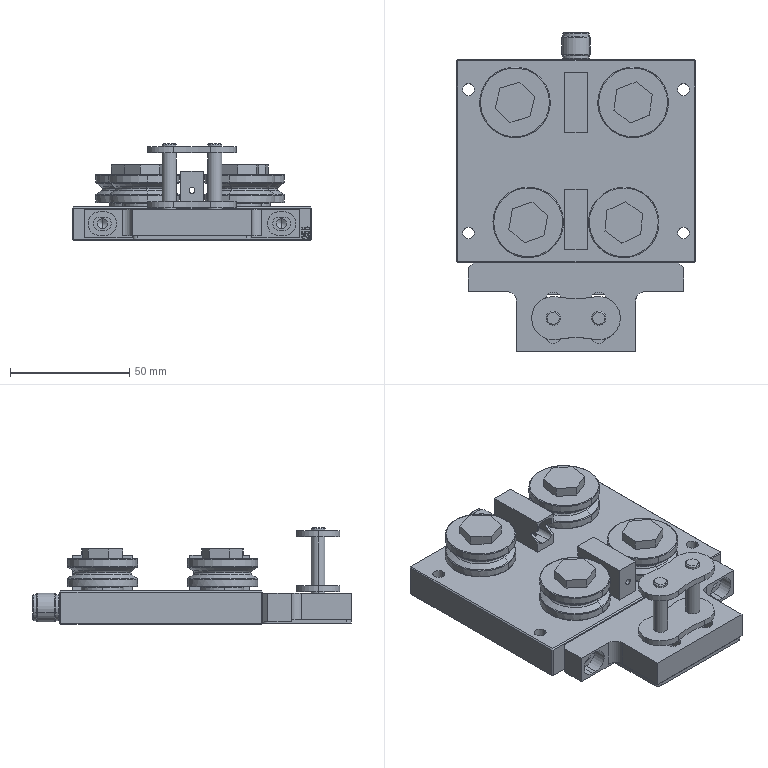Part | SolidWorks | features AEMSimFeature 1 | 29 solids | 918 faces | box 100 x 133.3 x 40.5 mm | volume 173730 mm3 | plane 416 | cylinder 290 | cone 76 | spline 72 | torus 64 | commonest cylinder face diameters 5 x34 6 x30 10 x30 2.5 x20 8 x18 13.7 x16